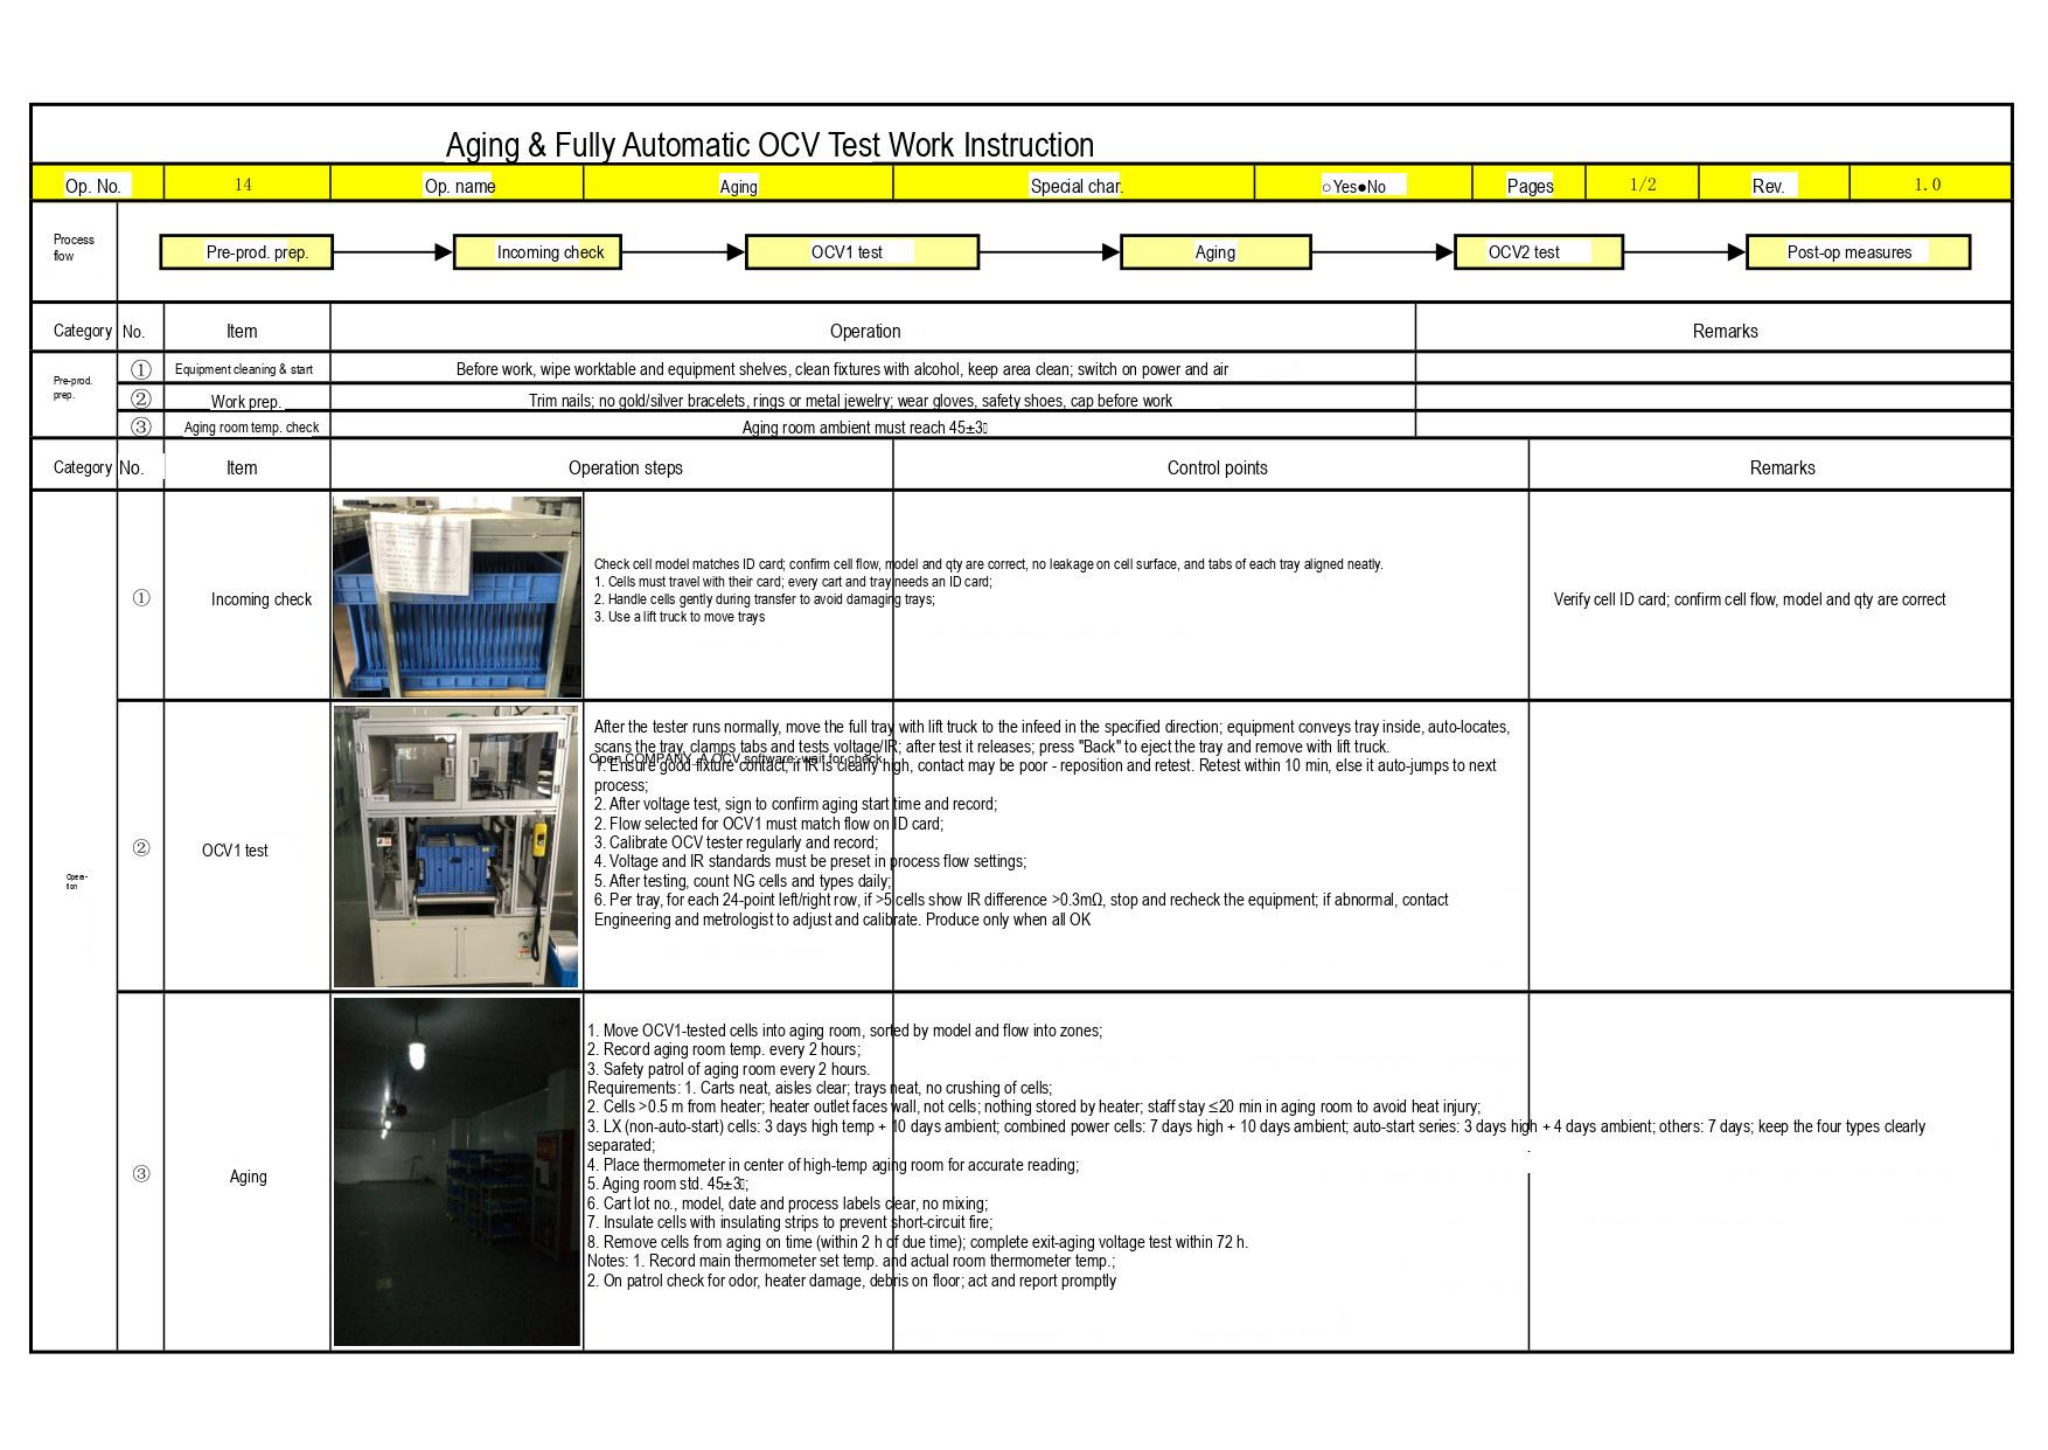# Aging & Fully Automatic OCV Test Work Instruction

| Op. No. | 14 | Op. name | Aging | Special char. | ○Yes●No | Pages | 1/2 | Rev. | 1.0 |
|---|---|---|---|---|---|---|---|---|---|

Process flow: Pre-prod. prep. → Incoming check → OCV1 test → Aging → OCV2 test → Post-op measures

| Category | No. | Item | Operation | Remarks |
|---|---|---|---|---|
| Pre-prod. prep. | ① | Equipment cleaning & start | Before work, wipe worktable and equipment shelves, clean fixtures with alcohol, keep area clean; switch on power and air | |
| | ② | Work prep. | Trim nails; no gold/silver bracelets, rings or metal jewelry; wear gloves, safety shoes, cap before work | |
| | ③ | Aging room temp. check | Aging room ambient must reach 45±3 | |

| Category | No. | Item | Operation steps | Control points | Remarks |
|---|---|---|---|---|---|
| Opera-tion | ① | Incoming check | Check cell model matches ID card; confirm cell flow, model and qty are correct, no leakage on cell surface, and tabs of each tray aligned neatly.<br>1. Cells must travel with their card; every cart and tray needs an ID card;<br>2. Handle cells gently during transfer to avoid damaging trays;<br>3. Use a lift truck to move trays | | Verify cell ID card; confirm cell flow, model and qty are correct |
| | ② | OCV1 test | After the tester runs normally, move the full tray with lift truck to the infeed in the specified direction; equipment conveys tray inside, auto-locates, scans the tray, clamps tabs and tests voltage/IR; after test it releases; press "Back" to eject the tray and remove with lift truck.<br>Open COMPANY_A OCV software, wait for check<br>1. Ensure good fixture contact; if IR is clearly high, contact may be poor - reposition and retest. Retest within 10 min, else it auto-jumps to next process;<br>2. After voltage test, sign to confirm aging start time and record;<br>2. Flow selected for OCV1 must match flow on ID card;<br>3. Calibrate OCV tester regularly and record;<br>4. Voltage and IR standards must be preset in process flow settings;<br>5. After testing, count NG cells and types daily;<br>6. Per tray, for each 24-point left/right row, if >5 cells show IR difference >0.3mΩ, stop and recheck the equipment; if abnormal, contact Engineering and metrologist to adjust and calibrate. Produce only when all OK | | |
| | ③ | Aging | 1. Move OCV1-tested cells into aging room, sorted by model and flow into zones;<br>2. Record aging room temp. every 2 hours;<br>3. Safety patrol of aging room every 2 hours.<br>Requirements: 1. Carts neat, aisles clear; trays neat, no crushing of cells;<br>2. Cells >0.5 m from heater; heater outlet faces wall, not cells; nothing stored by heater; staff stay ≤20 min in aging room to avoid heat injury;<br>3. LX (non-auto-start) cells: 3 days high temp + 10 days ambient; combined power cells: 7 days high + 10 days ambient; auto-start series: 3 days high + 4 days ambient; others: 7 days; keep the four types clearly separated;<br>4. Place thermometer in center of high-temp aging room for accurate reading;<br>5. Aging room std. 45±3;<br>6. Cart lot no., model, date and process labels clear, no mixing;<br>7. Insulate cells with insulating strips to prevent short-circuit fire;<br>8. Remove cells from aging on time (within 2 h of due time); complete exit-aging voltage test within 72 h.<br>Notes: 1. Record main thermometer set temp. and actual room thermometer temp.;<br>2. On patrol check for odor, heater damage, debris on floor; act and report promptly | | |
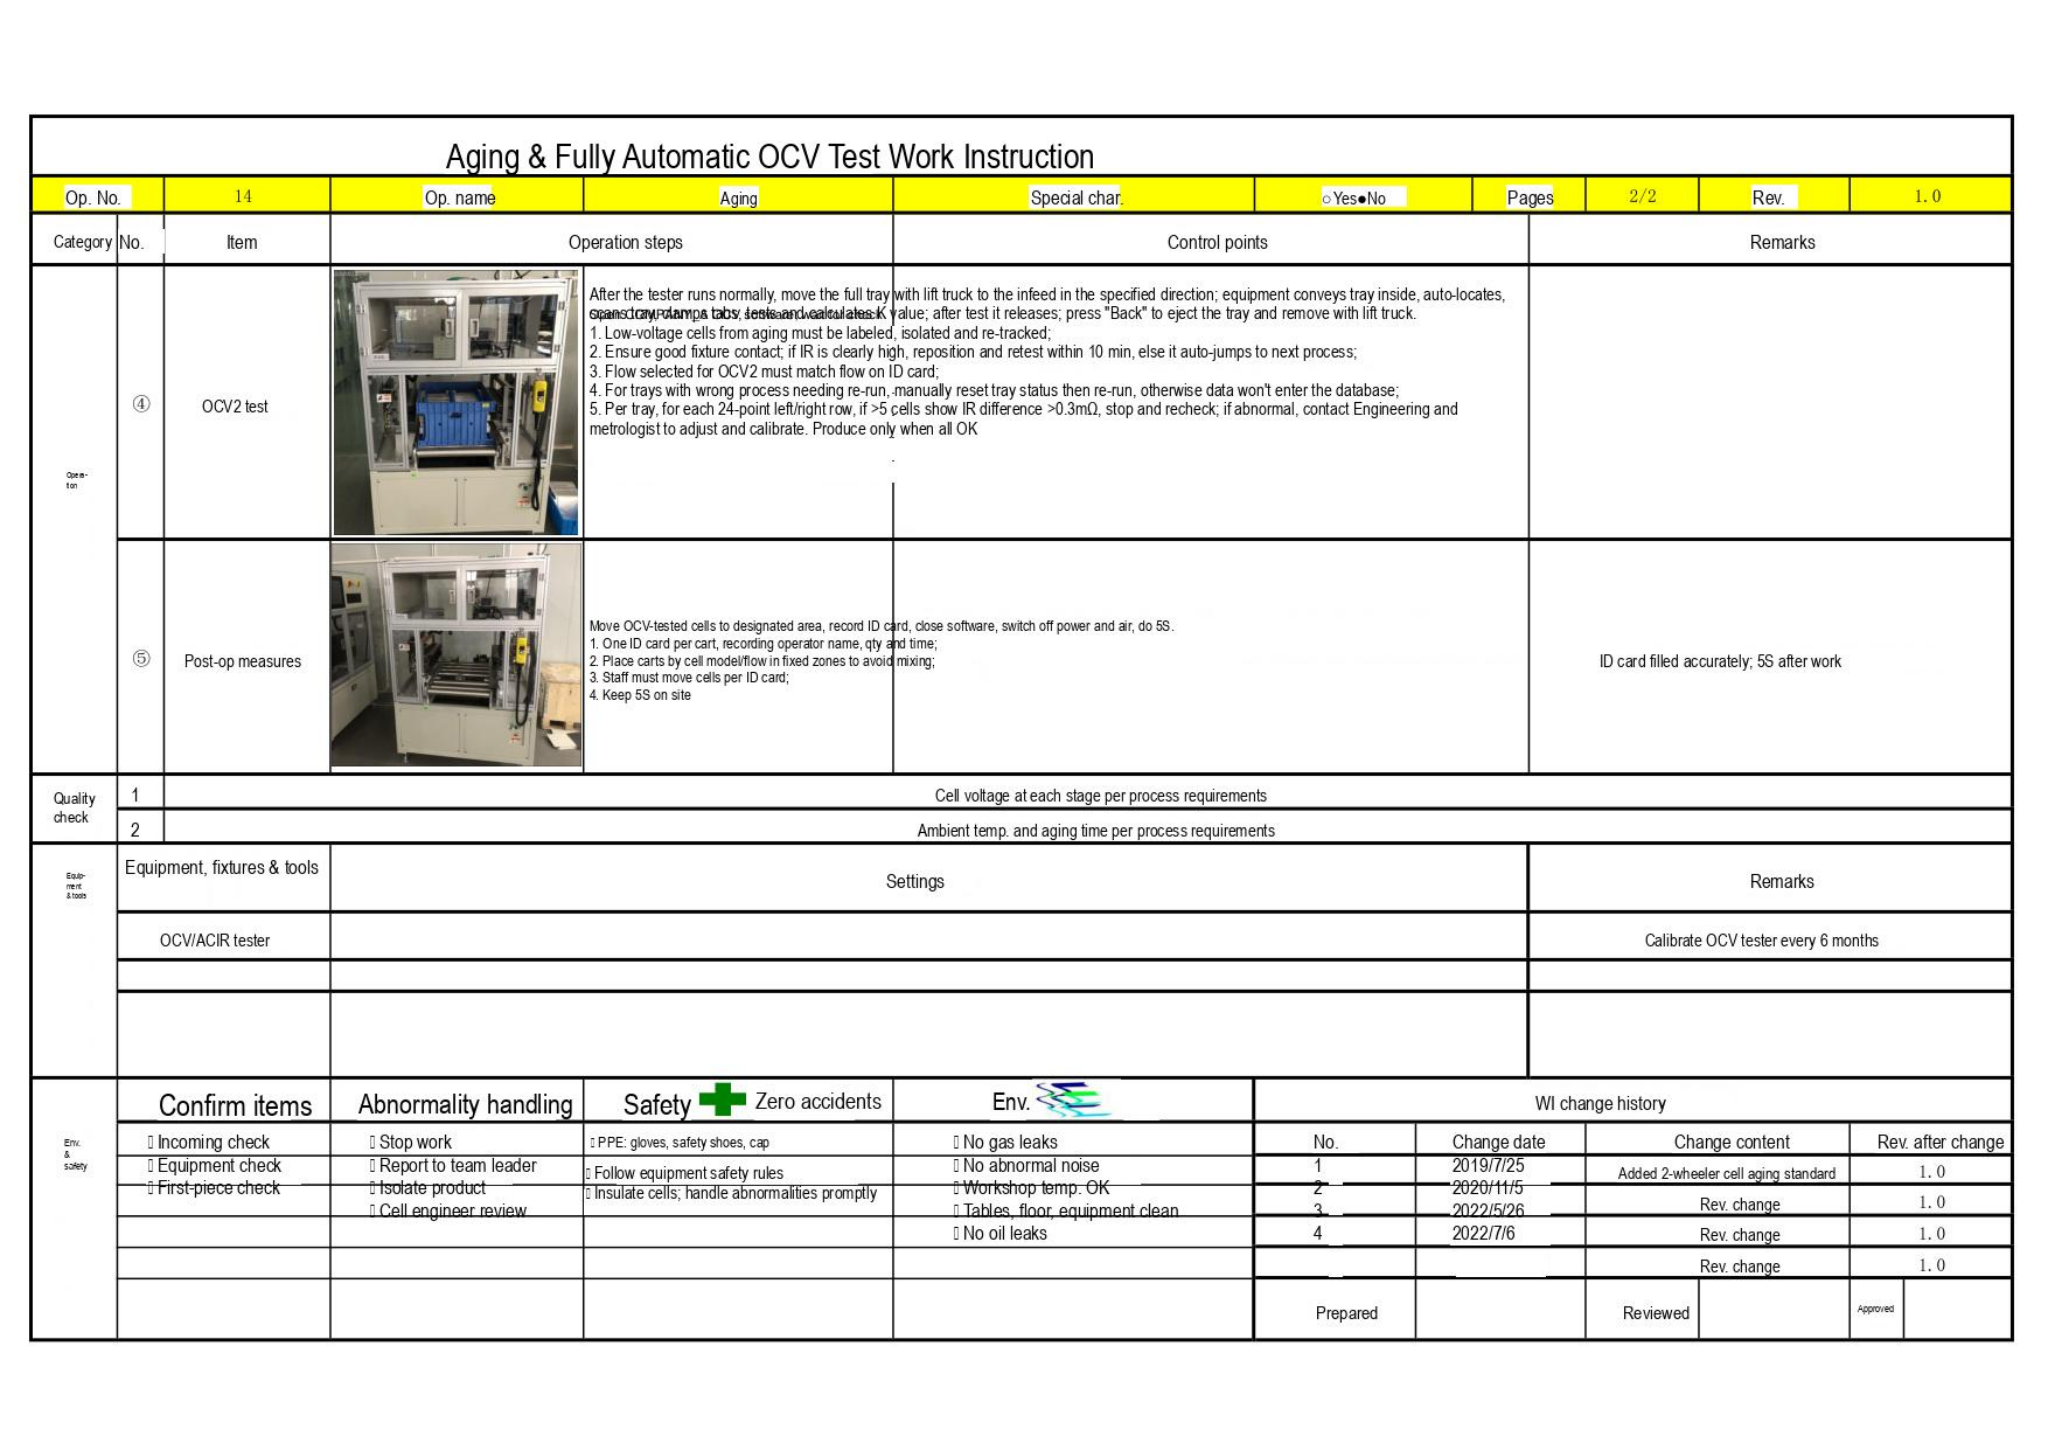# Aging & Fully Automatic OCV Test Work Instruction

| Op. No. | 14 | Op. name | Aging | Special char. | ○Yes●No | Pages | 2/2 | Rev. | 1.0 |
|---|---|---|---|---|---|---|---|---|---|

| Category | No. | Item | Operation steps | Control points | Remarks |
|---|---|---|---|---|---|
| Opera-tion | ④ | OCV2 test | After the tester runs normally, move the full tray with lift truck to the infeed in the specified direction; equipment conveys tray inside, auto-locates, clamps tabs, tests and calculates K value; after test it releases; press "Back" to eject the tray and remove with lift truck.<br>1. Low-voltage cells from aging must be labeled, isolated and re-tracked;<br>2. Ensure good fixture contact; if IR is clearly high, reposition and retest within 10 min, else it auto-jumps to next process;<br>3. Flow selected for OCV2 must match flow on ID card;<br>4. For trays with wrong process needing re-run, manually reset tray status then re-run, otherwise data won't enter the database;<br>5. Per tray, for each 24-point left/right row, if >5 cells show IR difference >0.3mΩ, stop and recheck; if abnormal, contact Engineering and metrologist to adjust and calibrate. Produce only when all OK | | |
| | ⑤ | Post-op measures | Move OCV-tested cells to designated area, record ID card, close software, switch off power and air, do 5S.<br>1. One ID card per cart, recording operator name, qty and time;<br>2. Place carts by cell model/flow in fixed zones to avoid mixing;<br>3. Staff must move cells per ID card;<br>4. Keep 5S on site | | ID card filled accurately; 5S after work |
| Quality check | 1 | Cell voltage at each stage per process requirements | | | |
| | 2 | Ambient temp. and aging time per process requirements | | | |

| Equip-ment & tools | Equipment, fixtures & tools | Settings | Remarks |
|---|---|---|---|
| | OCV/ACIR tester | | Calibrate OCV tester every 6 months |
| | | | |
| | | | |

| Env. & Safety | Confirm items | Abnormality handling | Safety Zero accidents | Env. |
|---|---|---|---|---|
| | Incoming check | Stop work | PPE: gloves, safety shoes, cap | No gas leaks |
| | Equipment check | Report to team leader | Follow equipment safety rules | No abnormal noise |
| | First-piece check | Isolate product | Insulate cells; handle abnormalities promptly | Workshop temp. OK |
| | | Cell engineer review | | Tables, floor, equipment clean |
| | | | | No oil leaks |

WI change history

| No. | Change date | Change content | Rev. after change |
|---|---|---|---|
| 1 | 2019/7/25 | Added 2-wheeler cell aging standard | 1.0 |
| 2 | 2020/11/5 | Rev. change | 1.0 |
| 3 | 2022/5/26 | Rev. change | 1.0 |
| 4 | 2022/7/6 | Rev. change | 1.0 |

| Prepared | | Reviewed | | Approved | |
|---|---|---|---|---|---|